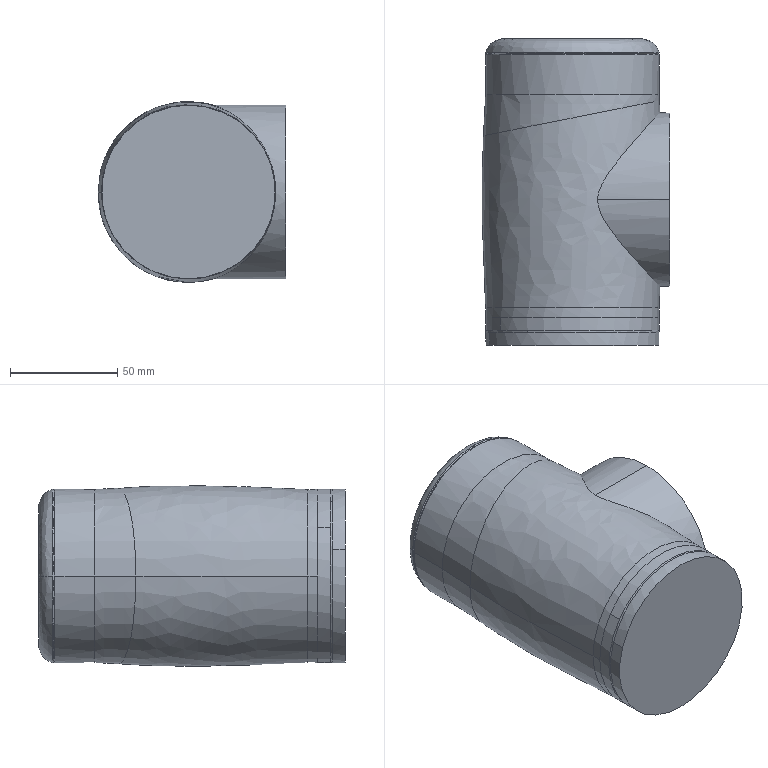Part | SolidWorks | features BaseBody 2 | 2 solids | 104 faces | box 87.688 x 143.092 x 84.375 mm | volume 806898 mm3 | cylinder 46 | plane 42 | torus 10 | spline 6 | commonest cylinder face diameters 0.4 x24 81 x12 47.7 x4 20 x2 20.6 x2 57 x2